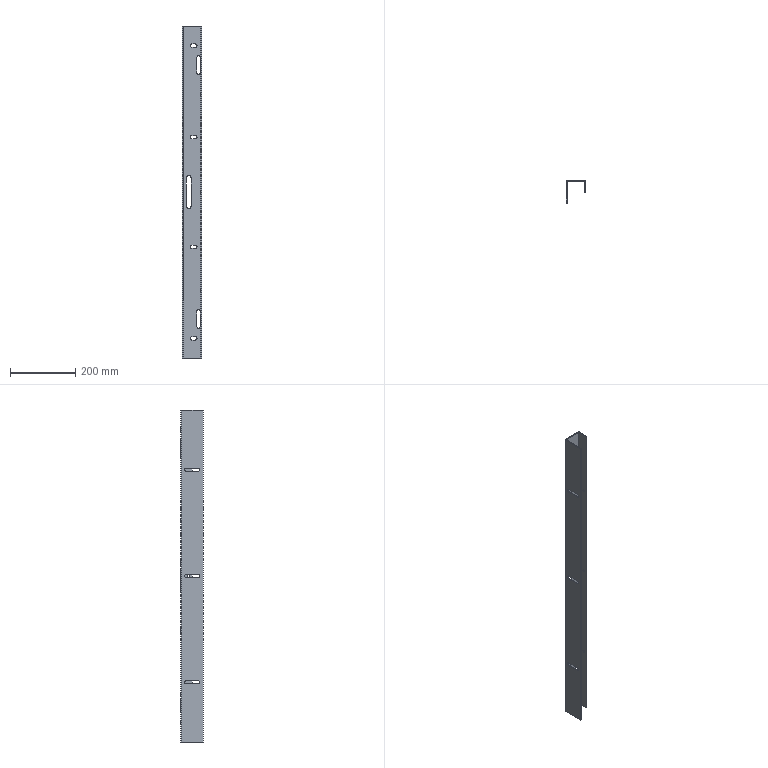Part | 1 solid | 74 faces | box 60 x 70 x 1015 mm | volume 465860 mm3 | plane 40 | cylinder 34 | commonest cylinder face diameters 10 x22 7 x6 0.2 x2 6.2 x2 14 x2